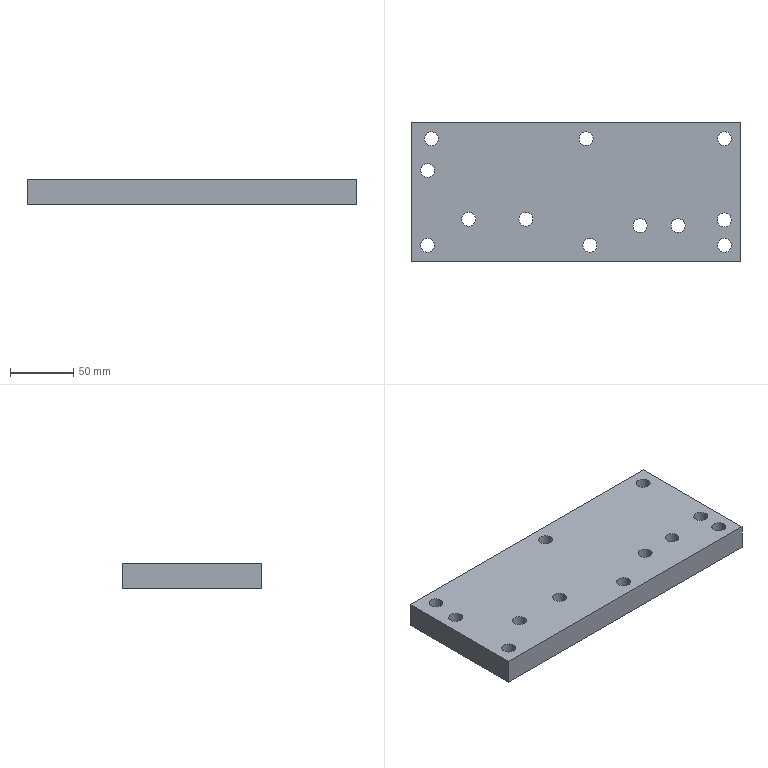Part | STEP file | 107_id3186_x_t | 1 solid | 18 faces | box 260 x 110 x 20 mm | volume 549192 mm3 | cylinder 12 | plane 6 | commonest cylinder face diameters 11 x12